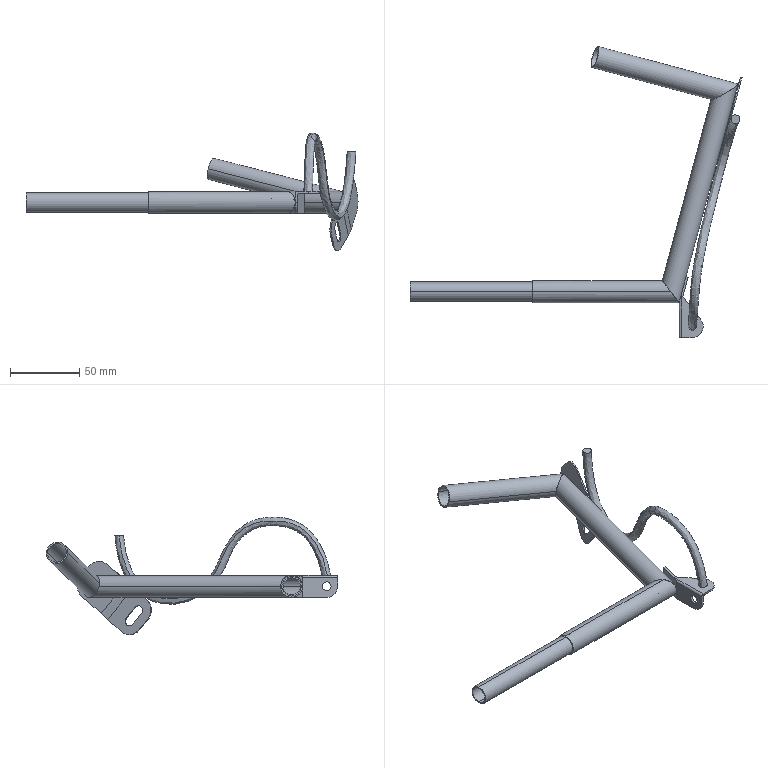Part | SolidWorks | features BaseBody 7 | 7 solids | 66 faces | box 240.534 x 211.019 x 85.41 mm | volume 31578 mm3 | cylinder 34 | plane 30 | spline 2 | commonest cylinder face diameters 14.097 x8 15.875 x8 20 x5 7 x3 3.048 x2 5.204 x2